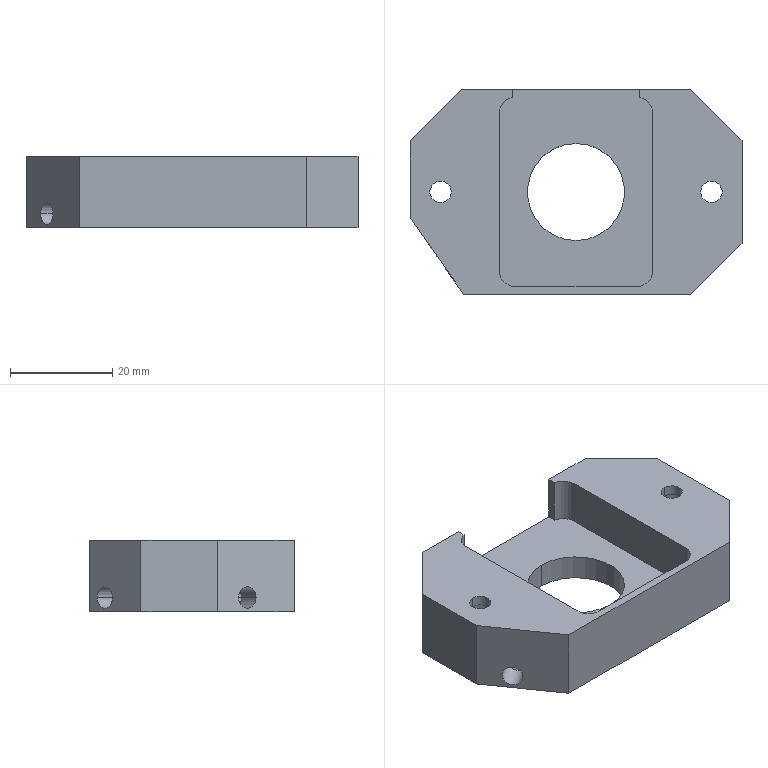NC program | NX | posted with a generic post | part box 65 x 40 x 14 mm
Whole program:
N10 G17 G21 G94 G90
(ADAPTIVE_MILLING_COPY_COPY_COPY , TOOL : D6)
N12 T06 M6
N14 G54
N16 G17 G0 G90 X10.343 Y12.642 S4500 M3
N18 G43 Z30. H6
N20 Z-7.85
N22 G94 G1 Z-8.85 F1000.
N24 X11.419 Y12.793 F1500.
N26 G3 X11.85 Y13.374 R0.611
N28 X9.957 Y15.33 R4.88
N30 G1 X9.945 Y15.334
N32 X9.933 Y15.337
N34 G3 X9.623 Y14.178 R0.701
N36 G1 Z-5.85
N38 G0 Z30.
N40 X10.691 Y13.063
N42 Z-7.85
N44 G1 Z-8.85 F1000.
N46 G3 X11.85 Y13.374 R0.69 F1500.
N48 X10.024 Y15.333 R3.971
N50 G1 X9.987 Y15.341
N52 X9.975 Y15.344
N54 X9.963 Y15.347
N56 X9.952 Y15.35
N58 X9.864
N60 G3 X9.399 Y14.222 R0.661
N62 G1 X10.804 Y12.838
N64 G3 X11.85 Y13.374 R0.661
N66 X10.094 Y15.336 R3.405
N68 G1 X10.057 Y15.344
N70 X10.045 Y15.346
N72 G3 X9.734 Y14.187 R0.704
N74 G1 Z-5.85
N76 G0 Z30.
N78 X10.691 Y13.075
N80 Z-7.85
N82 G1 Z-8.85 F1000.
N84 G3 X11.85 Y13.386 R0.63 F1500.
N86 X10.128 Y15.346 R2.898
N88 G1 X10.11 Y15.35
N90 X9.947
N92 G3 X9.472 Y14.232 R0.661
N94 G1 X10.793 Y12.872
N96 G3 X11.85 Y13.399 R0.661
N98 X10.722 Y15.093 R2.68
N100 X10.213 Y15.346 R2.465
N102 X9.902 Y14.187 R0.706
N104 G1 Z-5.85
N106 G0 Z30.
N108 X10.691 Y13.138
N110 Z-7.85
N112 G1 Z-8.85 F1000.
N114 G3 X11.85 Y13.449 R0.63 F1500.
N116 X10.297 Y15.346 R2.46
N118 X9.986 Y14.187 R0.706
N120 G1 Z-5.85
N122 G0 Z30.
N124 X10.691 Y13.188
N126 Z-7.85
N128 G1 Z-8.85 F1000.
N130 G3 X11.85 Y13.499 R0.63 F1500.
N132 X10.38 Y15.346 R2.299
N134 X10.07 Y14.187 R0.705
N136 G1 Z-5.85
N138 G0 Z30.
N140 X10.691 Y13.263
N142 Z-7.85
N144 G1 Z-8.85 F1000.
N146 G3 X11.85 Y13.574 R0.63 F1500.
N148 X10.442 Y15.35 R2.137
N150 G1 X10.105
N152 G3 X9.648 Y14.214 R0.661
N154 G1 X10.812 Y13.107
N156 G3 X11.85 Y13.649 R0.661
N158 X10.517 Y15.35 R1.998
N160 G1 X10.442
N162 G3 X9.92 Y14.286 R0.661
N164 G1 X10.742 Y13.239
N166 G3 X11.85 Y13.724 R0.661
N168 X10.589 Y15.35 R1.869
N170 G1 X10.514
N172 G3 X9.988 Y14.291 R0.661
N174 G1 X10.737 Y13.318
N176 G3 X11.85 Y13.799 R0.661
N178 X10.659 Y15.35 R1.747
N180 G1 X10.584
N182 G3 X10.054 Y14.296 R0.661
N184 G1 X10.728 Y13.402
N186 G3 X11.85 Y13.874 R0.661
N188 X10.726 Y15.35 R1.637
N190 G1 X10.651
N192 G3 X10.121 Y14.298 R0.661
N194 G1 X10.727 Y13.491
N196 G3 X11.85 Y13.961 R0.661
N198 X10.789 Y15.35 R1.529
N200 G1 X10.714
N202 G3 X10.181 Y14.302 R0.661
N204 G1 X10.724 Y13.569
N206 G3 X11.85 Y14.036 R0.661
N208 X10.785 Y15.35 R1.336
N210 X10.244 Y14.312 R0.661
N212 G1 X10.716 Y13.652
N214 G3 X11.85 Y14.111 R0.661
N216 X10.843 Y15.35 R1.25
N218 X10.299 Y14.316 R0.661
N220 G1 X10.712 Y13.731
N222 G3 X11.85 Y14.186 R0.661
N224 X10.895 Y15.35 R1.165
N226 X10.351 Y14.316 R0.661
N228 G1 X10.712 Y13.806
N230 G3 X11.85 Y14.261 R0.661
N232 X10.945 Y15.35 R1.087
N234 X10.396 Y14.323 R0.661
N236 G1 X10.706 Y13.874
N238 G3 X11.85 Y14.324 R0.661
N240 X11.004 Y15.35 R1.022
N242 X10.448 Y14.336 R0.661
N244 G1 X10.595 Y14.099
N246 X10.774 Y13.886
N248 G3 X11.85 Y14.399 R0.661
N250 X11.05 Y15.35 R0.953
N252 X10.487 Y14.346 R0.661
N254 G1 X10.611 Y14.141
N256 X10.765 Y13.956
N258 G3 X11.85 Y14.461 R0.661
N260 X11.09 Y15.35 R0.886
N262 X11.353 Y13.796 R-0.801
N264 X11.85 Y14.524 R0.787
N266 X11.139 Y15.35 R0.831
N268 X11.384 Y13.892 R-0.751
N270 X11.85 Y14.574 R0.737
N272 X11.174 Y15.35 R0.774
N274 X11.557 Y14.058 R-0.706
N276 X11.85 Y14.624 R0.704
N278 X11.206 Y15.35 R0.722
N280 X11.723 Y14.286 R-0.662
N282 X11.85 Y14.674 R0.7
N284 X11.231 Y15.35 R0.673
N286 X11.85 Y14.724 R-0.622
N288 X11.275 Y15.348 R0.63
N290 X11.736 Y14.413 R-0.598
N292 X11.846 Y14.806 R0.644
N294 X11.305 Y15.346 R0.618
N296 X10.696 Y14.959 R0.611
N298 G1 X10.261 Y13.827
N300 Z-5.85
N302 G0 Z30.
N304 X-9.143 Y13.842
N306 Z-7.85
N308 G1 Z-8.85 F1000.
N310 X-9.293 Y14.918 F1500.
N312 G3 X-9.874 Y15.35 R0.611
N314 X-11.83 Y13.457 R4.881
N316 G1 X-11.834 Y13.445
N318 X-11.837 Y13.433
N320 G3 X-10.678 Y13.123 R0.701
N322 G1 Z-5.85
N324 G0 Z30.
N326 X-9.563 Y14.191
N328 Z-7.85
N330 G1 Z-8.85 F1000.
N332 G3 X-9.874 Y15.35 R0.69 F1500.
N334 X-11.836 Y13.512 R3.892
N336 G1 X-11.838 Y13.499
N338 X-11.841 Y13.487
N340 X-11.844 Y13.475
N342 X-11.847 Y13.463
N344 X-11.85 Y13.452
N346 Y13.364
N348 G3 X-10.722 Y12.899 R0.661
N350 G1 X-9.338 Y14.304
N352 G3 X-9.874 Y15.35 R0.661
N354 X-11.841 Y13.569 R3.295
N356 G1 X-11.844 Y13.557
N358 X-11.846 Y13.545
N360 G3 X-10.687 Y13.234 R0.704
N362 G1 Z-5.85
N364 G0 Z30.
N366 X-9.575 Y14.191
N368 Z-7.85
N370 G1 Z-8.85 F1000.
N372 G3 X-9.886 Y15.35 R0.63 F1500.
N374 X-11.846 Y13.628 R2.898
N376 G1 X-11.85 Y13.61
N378 Y13.447
N380 G3 X-10.732 Y12.972 R0.661
N382 G1 X-9.372 Y14.293
N384 G3 X-9.899 Y15.35 R0.661
N386 X-11.585 Y14.232 R2.677
N388 X-11.85 Y13.607 R1.158
N390 X-10.756 Y13.11 R0.661
N392 G1 X-9.44 Y14.269
N394 G3 X-9.949 Y15.35 R0.661
N396 X-11.846 Y13.797 R2.461
N398 X-10.687 Y13.486 R0.706
N400 G1 Z-5.85
N402 G0 Z30.
N404 X-9.688 Y14.191
N406 Z-7.85
N408 G1 Z-8.85 F1000.
N410 G3 X-9.999 Y15.35 R0.63 F1500.
N412 X-11.85 Y13.861 R2.276
N414 G1 Y13.686
N416 G3 X-10.749 Y13.195 R0.661
N418 G1 X-9.559 Y14.276
N420 G3 X-10.074 Y15.35 R0.661
N422 X-11.85 Y13.942 R2.138
N424 G1 Y13.854
N426 G3 X-10.777 Y13.34 R0.661
N428 G1 X-9.657 Y14.25
N430 G3 X-10.149 Y15.35 R0.661
N432 X-11.85 Y14.016 R1.999
N434 G1 Y13.941
N436 G3 X-10.786 Y13.42 R0.661
N438 G1 X-9.739 Y14.242
N440 G3 X-10.224 Y15.35 R0.661
N442 X-11.85 Y14.089 R1.869
N444 G1 Y14.014
N446 G3 X-10.791 Y13.488 R0.661
N448 G1 X-9.818 Y14.237
N450 G3 X-10.299 Y15.35 R0.661
N452 X-11.85 Y14.158 R1.748
N454 G1 Y14.083
N456 G3 X-10.796 Y13.553 R0.661
N458 G1 X-9.902 Y14.228
N460 G3 X-10.374 Y15.35 R0.661
N462 X-11.85 Y14.226 R1.637
N464 G1 Y14.151
N466 G3 X-10.798 Y13.62 R0.661
N468 G1 X-9.991 Y14.227
N470 G3 X-10.461 Y15.35 R0.661
N472 X-11.85 Y14.289 R1.53
N474 G1 Y14.214
N476 G3 X-10.802 Y13.68 R0.661
N478 G1 X-10.069 Y14.224
N480 G3 X-10.536 Y15.35 R0.661
N482 X-11.85 Y14.284 R1.337
N484 X-10.811 Y13.744 R0.661
N486 G1 X-10.152 Y14.216
N488 G3 X-10.611 Y15.35 R0.661
N490 X-11.85 Y14.343 R1.251
N492 X-10.815 Y13.799 R0.661
N494 G1 X-10.23 Y14.213
N496 G3 X-10.686 Y15.35 R0.661
N498 X-11.85 Y14.394 R1.166
N500 X-10.815 Y13.851 R0.661
N502 G1 X-10.305 Y14.213
N504 G3 X-10.761 Y15.35 R0.661
N506 X-11.85 Y14.445 R1.088
N508 X-10.823 Y13.896 R0.661
N510 G1 X-10.374 Y14.207
N512 G3 X-10.824 Y15.35 R0.661
N514 X-11.85 Y14.504 R1.023
N516 X-10.835 Y13.948 R0.661
N518 G1 X-10.599 Y14.095
N520 X-10.386 Y14.274
N522 G3 X-10.899 Y15.35 R0.661
N524 X-11.85 Y14.55 R0.953
N526 X-10.846 Y13.987 R0.661
N528 G1 X-10.64 Y14.112
N530 X-10.455 Y14.266
N532 G3 X-10.961 Y15.35 R0.661
N534 X-11.85 Y14.589 R0.887
N536 X-10.296 Y14.853 R-0.801
N538 X-11.024 Y15.35 R0.787
N540 X-11.85 Y14.639 R0.831
N542 X-10.392 Y14.884 R-0.751
N544 X-11.074 Y15.35 R0.737
N546 X-11.85 Y14.673 R0.774
N548 X-10.558 Y15.057 R-0.706
N550 X-11.124 Y15.35 R0.704
N552 X-11.85 Y14.705 R0.722
N554 X-10.786 Y15.223 R-0.662
N556 X-11.174 Y15.35 R0.7
N558 X-11.85 Y14.731 R0.673
N560 X-11.224 Y15.35 R-0.622
N562 X-11.848 Y14.775 R0.631
N564 X-10.913 Y15.236 R-0.598
N566 X-11.306 Y15.346 R0.644
N568 X-11.846 Y14.805 R0.618
N570 X-11.459 Y14.196 R0.611
N572 G1 X-10.326 Y13.761
N574 Z-5.85
N576 G0 Z30.
N578 X-10.349 Y-13.386
N580 Z-7.85
N582 G1 Z-8.85 F1000.
N584 X-11.419 Y-13.537 F1500.
N586 G3 X-11.85 Y-14.117 R0.611
N588 X-10.916 Y-15.765 R16.455
N590 G1 X-10.897 Y-15.782
N592 X-10.878 Y-15.798
N594 X-10.864 Y-15.81
N596 X-10.858 Y-15.813
N598 X-10.844 Y-15.824
N600 X-10.487 Y-16.136
N602 G3 X-9.524 Y-15.245 R0.66
N604 G1 X-10.729 Y-13.645
N606 G3 X-11.85 Y-14.117 R0.661
N608 X-10.963 Y-15.751 R4.717
N610 G1 X-10.933 Y-15.773
N612 X-10.923 Y-15.781
N614 X-10.905 Y-15.793
N616 X-10.873 Y-15.806
N618 X-10.862 Y-15.811
N620 G3 X-10.006 Y-14.893 R0.66
N622 G1 X-10.673 Y-13.707
N624 G3 X-11.85 Y-14.117 R0.661
N626 X-10.981 Y-15.763 R2.978
N628 G1 X-10.899 Y-15.796
N630 G3 X-10.067 Y-14.883 R0.661
N632 G1 X-10.656 Y-13.743
N634 G3 X-11.85 Y-14.13 R0.66
N636 X-11.058 Y-15.733 R2.475
N638 G1 X-10.977 Y-15.765
N640 G3 X-10.133 Y-14.876 R0.661
N642 G1 X-10.641 Y-13.788
N644 G3 X-11.85 Y-14.155 R0.66
N646 X-11.136 Y-15.701 R2.145
N648 G1 X-11.055 Y-15.734
N650 G3 X-10.204 Y-14.862 R0.661
N652 G1 X-10.632 Y-13.877
N654 G3 X-11.85 Y-14.23 R0.66
N656 X-11.236 Y-15.652 R1.914
N658 X-10.387 Y-14.803 R0.713
N660 G1 Z-5.85
N662 G0 Z30.
N664 X-10.65 Y-14.355
N666 Z-7.85
N668 G1 Z-8.85 F1000.
N670 G3 X-11.85 Y-14.355 R0.601 F1500.
N672 X-11.277 Y-15.646 R1.64
N674 G1 X-11.126 Y-15.706
N676 G3 X-10.292 Y-14.796 R0.661
N678 G1 X-10.654 Y-14.095
N680 G3 X-11.85 Y-14.48 R0.66
N682 X-11.367 Y-15.599 R1.451
N684 X-10.519 Y-14.75 R0.746
N686 G1 Z-5.85
N688 G0 Z30.
N690 X-10.691 Y-14.282
N692 Z-7.85
N694 G1 Z-8.85 F1000.
N696 G3 X-11.85 Y-14.592 R0.63 F1500.
N698 X-11.276 Y-15.646 R1.063
N700 X-10.438 Y-14.746 R0.661
N702 G1 X-10.559 Y-14.487
N704 X-10.714 Y-14.248
N706 G3 X-11.85 Y-14.705 R0.661
N708 X-11.382 Y-15.604 R0.966
N710 X-10.5 Y-14.825 R0.661
N712 X-10.7 Y-14.35 R1.037
N714 X-11.85 Y-14.792 R0.661
N716 X-11.433 Y-15.584 R0.847
N718 X-11.162 Y-14.166 R-0.737
N720 X-11.85 Y-14.88 R0.718
N722 X-11.483 Y-15.563 R0.742
N724 G1 X-10.887 Y-15.636
N726 G3 X-10.356 Y-14.517 R0.653
N728 X-11.674 Y-14.531 R0.9
N730 X-11.518 Y-15.546 R0.653
N732 X-11.847 Y-15.056 R-0.583
N734 X-11.576 Y-15.512 R0.694
N736 X-10.722 Y-15.309 R0.609
N738 G1 X-10.225 Y-14.457
N740 Z-5.85
N742 G0 Z30.
N744 X8.928 Y-15.536
N746 Z-7.85
N748 G1 Z-8.85 F1000.
N750 X9.8 Y-16.213 F1500.
N752 G3 X10.487 Y-16.136 R0.613
N754 X11.255 Y-15.166 R2.944
N756 X11.85 Y-14.105 R2.583
N758 X10.636 Y-13.746 R0.66
N760 G1 X9.778 Y-15.085
N762 G3 X10.816 Y-15.848 R0.66
N764 X11.85 Y-14.263 R4.647
N766 G1 Y-14.163
N768 G3 X10.643 Y-13.794 R0.66
N770 G1 X9.801 Y-15.058
N772 G3 X10.835 Y-15.832 R0.66
N774 X11.843 Y-14.406 R3.545
N776 X10.684 Y-14.096 R0.71
N778 G1 Z-5.85
N780 G0 Z30.
N782 X10.009 Y-14.965
N784 Z-7.85
N786 G1 Z-8.85 F1000.
N788 G3 X10.858 Y-15.813 R0.636 F1500.
N790 X11.85 Y-14.479 R2.656
N792 G1 Y-14.254
N794 G3 X10.633 Y-13.9 R0.66
N796 G1 X9.973 Y-14.954
N798 G3 X10.858 Y-15.813 R0.661
N800 X11.85 Y-14.475 R1.839
N802 X10.67 Y-14.069 R0.661
N804 G1 X10.05 Y-14.876
N806 G3 X10.873 Y-15.806 R0.661
N808 X11.85 Y-14.566 R1.607
N810 X10.683 Y-14.144 R0.661
N812 G1 X10.118 Y-14.836
N814 G3 X10.931 Y-15.783 R0.661
N816 X11.85 Y-14.662 R1.437
N818 X10.696 Y-14.224 R0.661
N820 G1 X10.213 Y-14.782
N822 G3 X11.013 Y-15.75 R0.66
N824 X11.85 Y-14.745 R1.276
N826 X10.71 Y-14.292 R0.661
N828 G1 X10.304 Y-14.734
N830 G3 X11.094 Y-15.718 R0.66
N832 X11.85 Y-14.814 R1.123
N834 X10.723 Y-14.347 R0.661
N836 G1 X10.517 Y-14.549
N838 X10.341 Y-14.778
N840 G3 X11.175 Y-15.686 R0.661
N842 X11.85 Y-14.887 R0.997
N844 X10.758 Y-14.388 R0.661
N846 X10.396 Y-14.806 R1.097
N848 X11.257 Y-15.654 R0.661
N850 X11.85 Y-14.956 R0.886
N852 X10.396 Y-15.236 R-0.755
N854 X11.338 Y-15.621 R0.737
N856 X11.85 Y-15.011 R0.779
N858 G1 X11.698 Y-14.431
N860 G3 X10.431 Y-14.343 R0.671
N862 X10.937 Y-15.591 R0.917
N864 X11.846 Y-15.061 R0.68
N866 X11.104 Y-15.604 R-0.606
N868 X11.49 Y-15.559 R0.643
N870 X11.836 Y-15.128 R0.677
N872 X11.245 Y-14.403 R0.608
N874 G1 X10.329 Y-14.398
N876 Z-5.85
N878 G0 Z30.
N880 M5
(11_COPY_COPY_COPY_COPY_COPY_1 , TOOL : D6A45)
N882 T01 M6
N884 G54
N886 G17 G0 G90 X-27.641 Y0. S7500 M3
N888 G43 Z30. H1
N890 Z3.
N892 G94 G1 Z-1. F1000.
N894 G3 X-26.5 Y-1.141 R1.141
N896 X-27.641 Y0. R-1.141
N898 X-27.341 Y-0.52 R0.6
N900 G1 Z2.
N902 G0 Z30.
N904 X27.641 Y0.
N906 Z3.
N908 G1 Z-1.
N910 G3 X26.5 Y1.141 R1.141
N912 X27.641 Y0. R-1.141
N914 X27.341 Y0.52 R0.6
N916 G1 Z2.
N918 G0 Z30.
N920 X-23.421 Y21.952
N922 Z2.
N924 G1 Z-1.
N926 X-23.02 Y21.259
N928 G3 X-22.501 Y20.959 R0.6
N930 G1 X21.998
N932 G2 X22.782 Y20.55 R0.957
N934 G1 X33.286 Y5.549
N936 G2 X33.459 Y5.001 R0.956
N938 G1 Y-10.001
N940 G2 X33.179 Y-10.677 R0.956
N942 G1 X23.177 Y-20.678
N944 G2 X22.501 Y-20.959 R0.957
N946 G1 X12.499
N948 G2 X11.541 Y-20.001 R0.958
N950 G1 Y-18.499
N952 G2 X12.348 Y-17.554 R0.965
N954 G3 X14.041 Y-15.542 R2.041
N956 G1 Y15.5
N958 G3 X12. Y17.541 R2.041
N960 G1 X-12.
N962 G3 X-14.041 Y15.5 R2.041
N964 G1 Y-15.542
N966 G3 X-12.34 Y-17.555 R2.041
N968 G2 X-11.541 Y-18.499 R0.958
N970 G1 Y-20.001
N972 G2 X-12.499 Y-20.959 R0.958
N974 G1 X-22.501
N976 G2 X-23.177 Y-20.678 R0.957
N978 G1 X-33.179 Y-10.677
N980 G2 X-33.459 Y-10.001 R0.956
N982 G1 Y10.001
N984 G2 X-33.179 Y10.677 R0.956
N986 G1 X-23.177 Y20.678
N988 G2 X-22.501 Y20.959 R0.957
N990 G3 X-21.981 Y21.259 R0.6
N992 G1 X-21.461 Y22.159
N994 Z2.
N996 G0 Z30.
N998 M5
N1000 M2